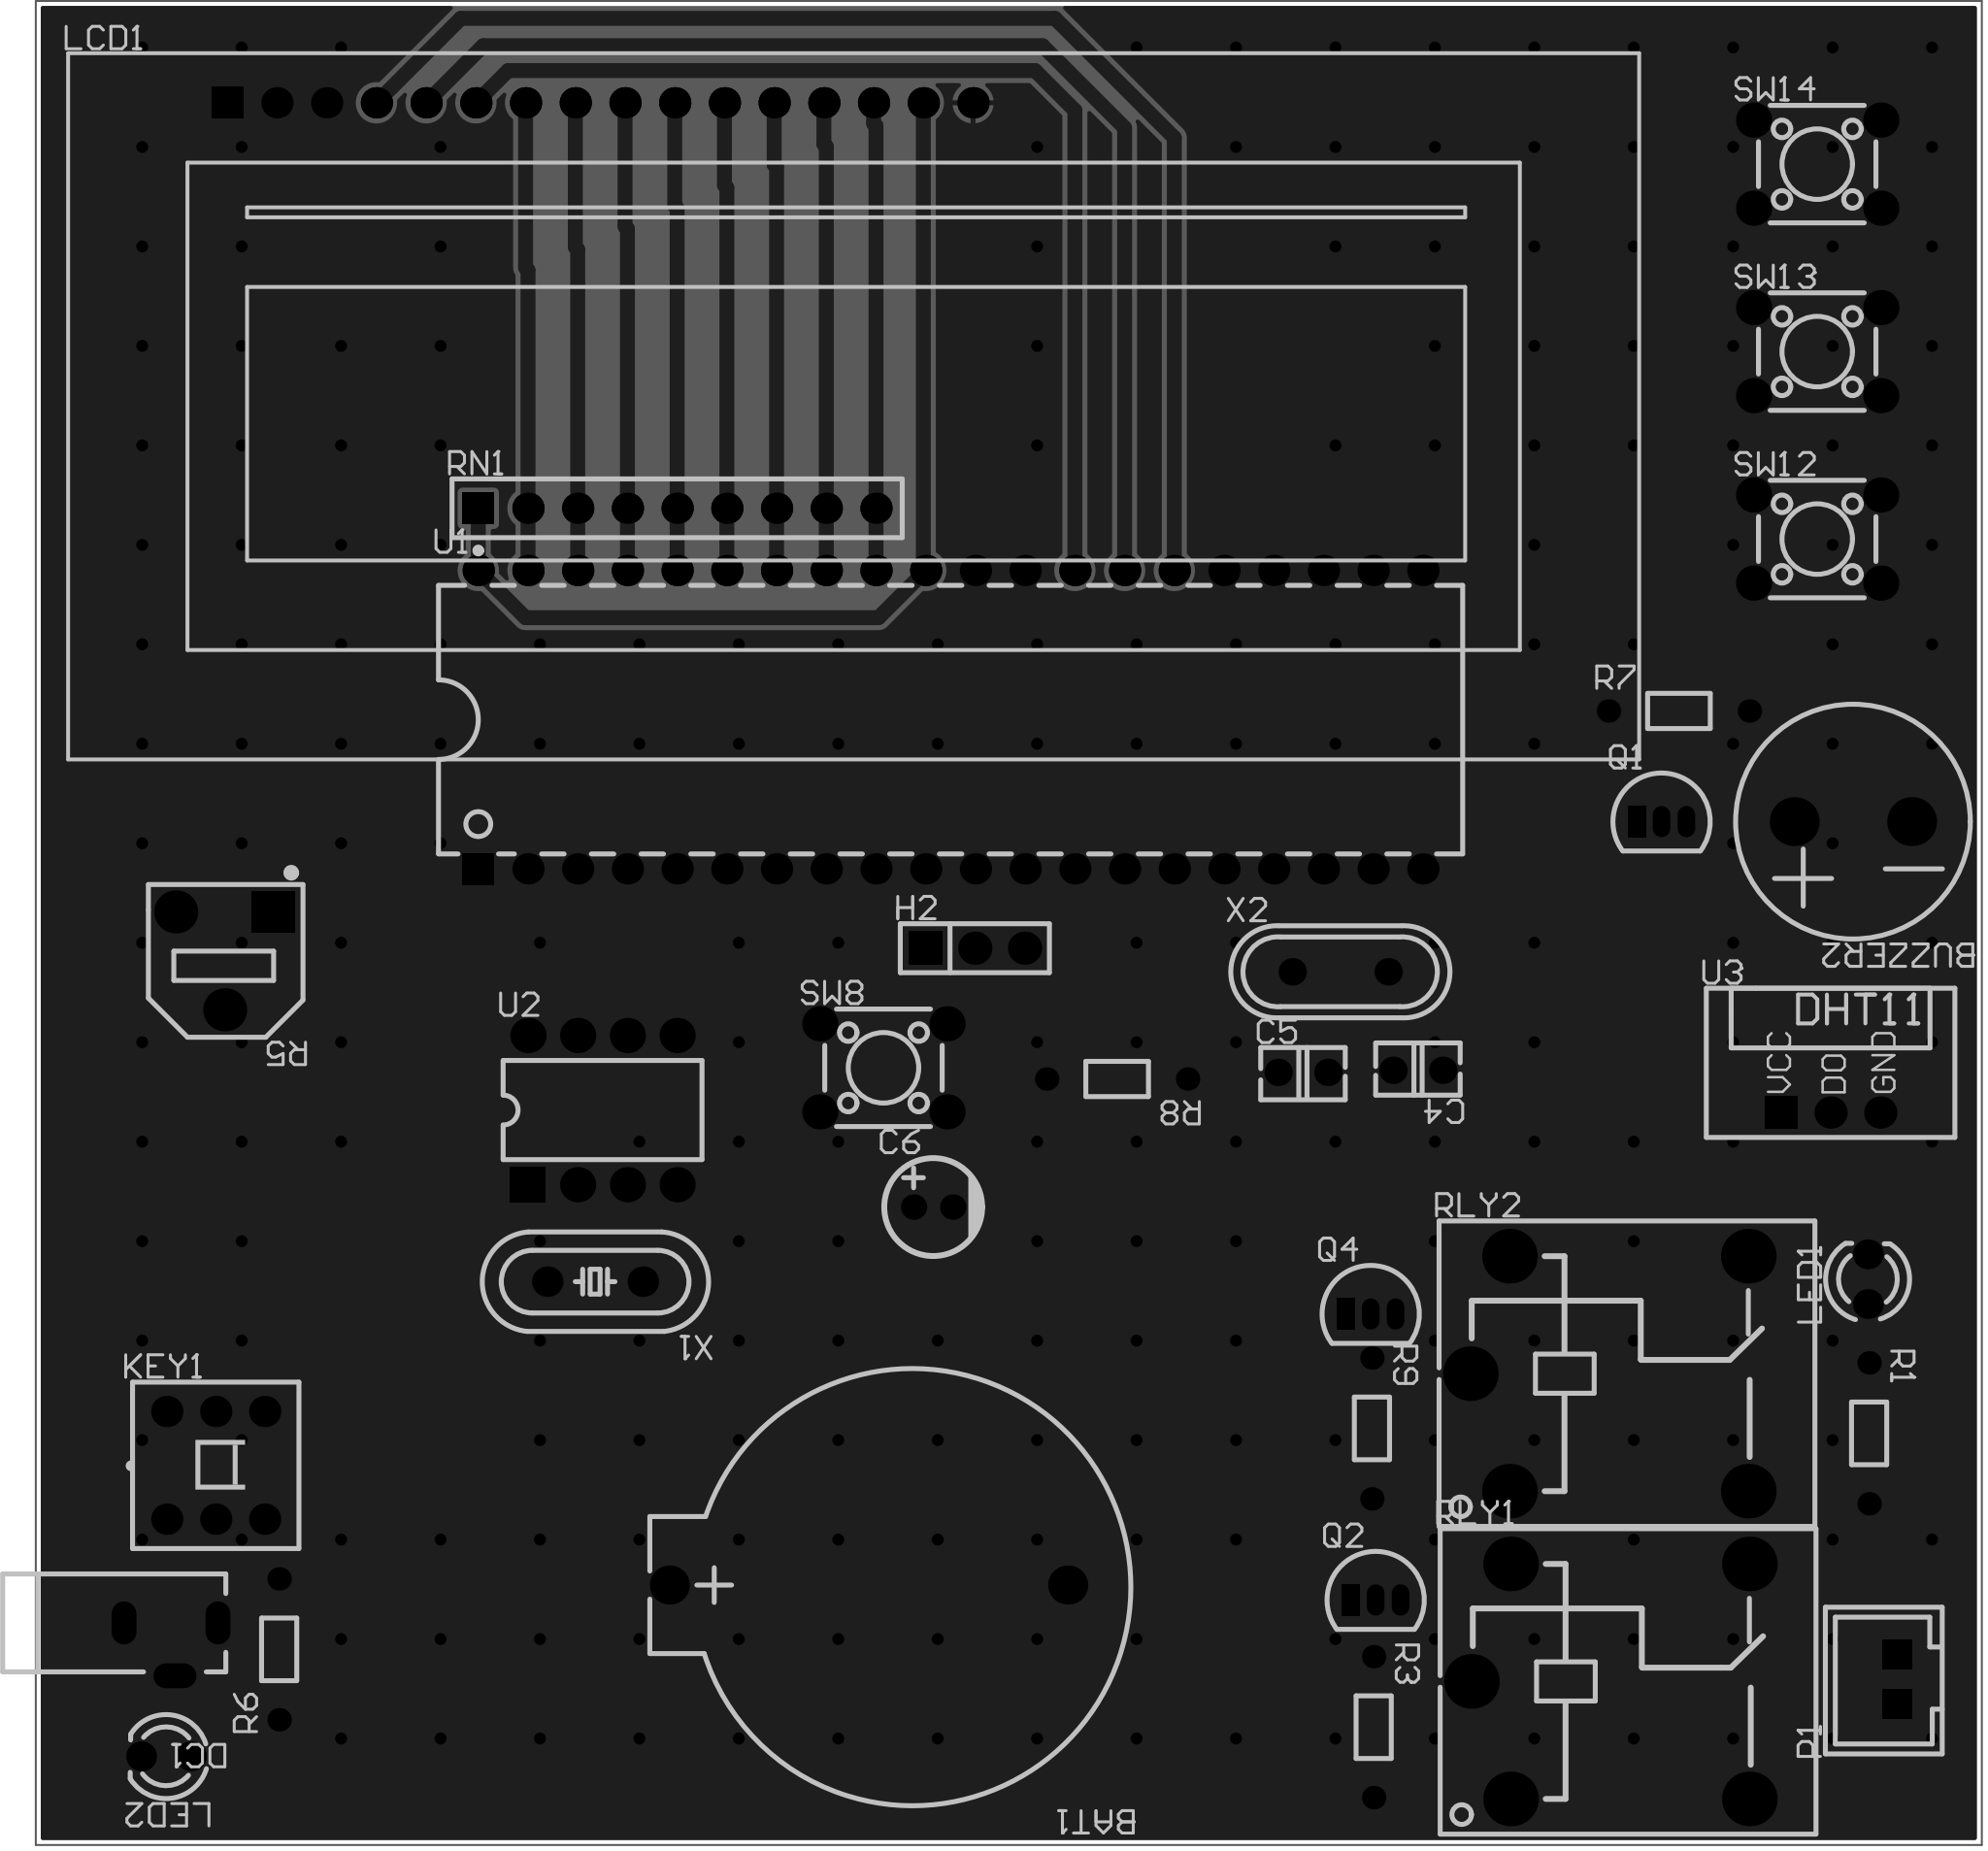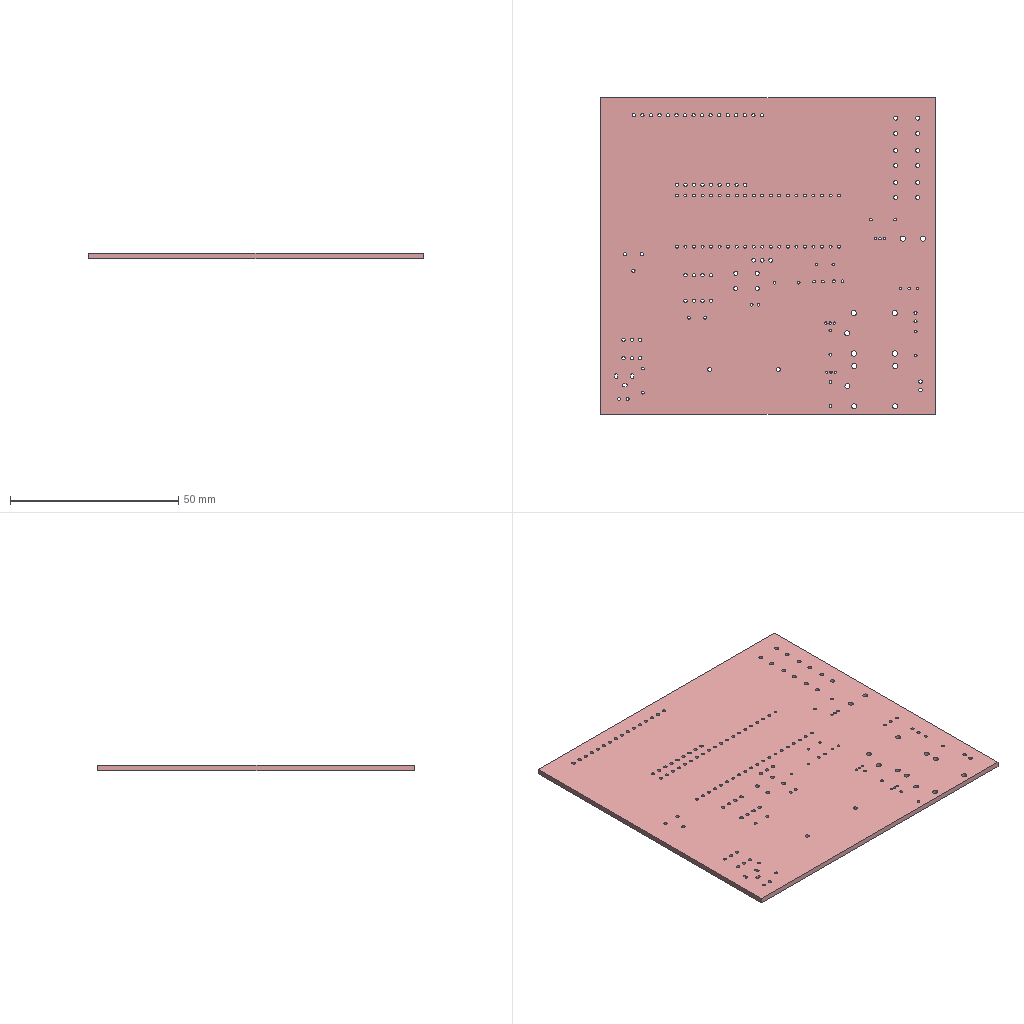Circuit board layout | Altium Designer | box 99.4 x 94.2 x 1.6 mm
Layer stack:
# Altium Designer layer stack of  (unit mm; dielectric type: 0 none, 1 core, 2 prepreg, 3 surface material)
index,name,kind,layer,copper_thickness_mm,dielectric_type,dielectric_thickness_mm,dielectric_material,dielectric_constant
0,Top Paste Mask Layer,other,,,,,,
1,Top Silkscreen Layer,other,,,,,,
2,Top Solder Mask Layer,dielectric,,,3,0.01,,3.3
3,Top Layer,copper,Top Layer,0.035,,,,
4,Dielectric1,dielectric,,,3,1.51,FR4,4.5
5,Bottom Layer,copper,Bottom Layer,0.035,,,,
6,Bottom Solder Mask Layer,dielectric,,,3,0.01,,3.3
7,Bottom Silkscreen Layer,other,,,,,,
8,Bottom Paste Mask Layer,other,,,,,,
# drill layer pairs: low layer,high layer
drill_pair,Top Layer,Bottom Layer
Part placement:
Designator,Comment,Layer,Footprint,Center-X(mm),Center-Y(mm),Rotation
BUZZER2,buzzer,TopLayer,BUZ-TH_BD12.0-P6.00-D0.9-RD,177.546,140.081,180
C4,30pF,TopLayer,CAP-TH_L3.8-W2.5-P2.54-D0.50,155.321,127.381,180
C5,30pF,TopLayer,CAP-TH_L3.8-W2.5-P2.54-D0.50,149.449,127.272,0
C6,10uF,TopLayer,CAP-TH_BD5.0-P2.00-D0.8-FD-10UF50VC110GL,130.556,120.396,0
H2,,TopLayer,HDR-TH_3P-P2.54-V-M,132.685,133.616,0
KEY1,无自锁开关 8.5×8.5 无声,TopLayer,SW-TH_6P-L8.5-W8.5-P2.54,93.903,107.206,0
LCD1,LCD1602,TopLayer,LCD1602,113.542,176.79,0
LED2,,TopLayer,LED_TH-3mm,91.363,92.347,180
Q4,,TopLayer,S8550P_TO-92,152.908,114.935,0
R7,300Ω,TopLayer,Res_1/8W,168.656,145.732,0
R8,10kΩ,TopLayer,Res_1/8W,139.954,126.937,180
R9,1kΩ,TopLayer,Res_1/8W,152.971,109.093,270
R5,10kΩ,TopLayer,RES-ADJ-SMD_RM065-V1,94.361,132.969,180
R6,1kΩ,TopLayer,Res_1/8W,97.142,97.808,90
RLY2,SRD-05VDC-SL-C,TopLayer,RELAY-TH_SRD-XXVDC-XL-C,165.1,111.887,0
SW8,,TopLayer,SW-TH_4P-L6.0-W6.0-P4.50-LS6.5,128.016,127.508,0
SW12,,TopLayer,SW-TH_4P-L6.0-W6.0-P4.50-LS6.5,175.72,154.511,0
SW13,,TopLayer,SW-TH_4P-L6.0-W6.0-P4.50-LS6.5,175.72,164.084,0
SW14,,TopLayer,SW-TH_4P-L6.0-W6.0-P4.50-LS6.5,175.72,173.657,0
U1,STC89C52RC-40I-PDIP40,TopLayer,DIP-40_L52.0-W13.7-P2.54-LS15.2-BL,131.445,145.288,0
X2,11.059MHz,TopLayer,OSC-TH_L11.1-W4.7-P4.88,151.354,132.411,0
DC1,DC-002,TopLayer,DC-IN-TH_DC-3510,91.617,97.808,180
RN1,-,TopLayer,RES-ARRAY-TH_9P-P2.54-D1.0,117.475,156.083,0
BAT1,CR2032-2-1,TopLayer,BAT-TH_CR2032-2-1,127.254,101.092,180
LED1,,TopLayer,LED_TH-3mm,178.308,116.713,90
P1,XH2.54直插座-2P,TopLayer,CONN-TH_XH2.54-2P,179.82,96.277,90
Q2,,TopLayer,S8550P_TO-92,153.162,100.33,0
R1,300Ω,TopLayer,Res_1/8W,178.371,108.839,270
R3,1kΩ,TopLayer,Res_1/8W,153.06,93.835,270
RLY1,SRD-05VDC-SL-C,TopLayer,RELAY-TH_SRD-XXVDC-XL-C,165.155,96.17,0
U2,DS1302N,TopLayer,DIP-8_L9.7-W6.4-P2.54-LS7.6-BL,113.665,125.349,0
U3,DHT11,TopLayer,DHT11_X,176.403,125.222,0
X1,32.768HZ,TopLayer,HC-49S_L11.5-W5.0-P4.88,113.284,116.586,180
Q1,,TopLayer,S8550P_TO-92,167.767,140.081,0
Pad and via stacks:
# Altium Designer via and pad stacks of  (unit mm). Each distinct definition once, with the count of objects using it.
# via: kind,start_layer,end_layer,hole_mm,diameter_mm,mode(0 simple;1 top-mid-bottom;2 full stack),diameter_per_layer,count,example_net
# pad: kind,layer,hole_mm,hole_type(0 round;1 square;2 slot),plating,top_size,top_shape(1 round;2 rect;3 octagon;9 rounded rect),mid_size,bottom_size,mode,footprint,size_per_layer,count,example
pad,Multi-Layer,1.5,0,plated,2.5x2.5,1,2.5x2.5,2.5x2.5,0,BUZ-TH_BD12.0-P6.00-D0.9-RD,,2,BUZZER2.1
pad,Multi-Layer,0.8,0,plated,1.4x1.4,1,1.4x1.4,1.4x1.4,0,CAP-TH_L3.8-W2.5-P2.54-D0.50,,4,C4.1
pad,Multi-Layer,0.8,0,plated,1.3x1.3,1,1.3x1.3,1.3x1.3,0,CAP-TH_BD5.0-P2.00-D0.8-FD-10UF50VC110GL,,2,C6.2
pad,Multi-Layer,1.1,0,plated,1.7x1.7,2,1.7x1.7,1.7x1.7,0,HDR-TH_3P-P2.54-V-M,,1,H2.1
pad,Multi-Layer,1.1,0,plated,1.7x1.7,1,1.7x1.7,1.7x1.7,0,HDR-TH_3P-P2.54-V-M,,2,H2.2
pad,Multi-Layer,1,0,plated,1.6x1.6,1,1.6x1.6,1.6x1.6,0,SW-TH_6P-L8.5-W8.5-P2.54,,6,KEY1.4
pad,Multi-Layer,1,0,plated,1.6x1.6,1,1.6x1.6,1.6x1.6,0,LCD1602,,15,LCD1.16
pad,Multi-Layer,1,0,plated,1.6x1.6,2,1.6x1.6,1.6x1.6,0,LCD1602,,1,LCD1.1
pad,Multi-Layer,0.9144,0,plated,1.524x1.524,1,1.524x1.524,1.524x1.524,0,LED_TH-3mm,,4,LED2.1
pad,Multi-Layer,0.7,0,plated,0.9x1.6,1,0.9x1.6,0.9x1.6,0,S8550P_TO-92,,6,Q4.3
pad,Multi-Layer,0.7,0,plated,0.9x1.6,2,0.9x1.6,0.9x1.6,0,S8550P_TO-92,,3,Q4.1
pad,Multi-Layer,0.8001,0,plated,1.199x1.199,1,1.199x1.199,1.199x1.199,0,Res_1/8W,,12,R7.1
pad,Multi-Layer,1,0,plated,2.2x2.1,2,2.2x2.1,2.2x2.1,0,RES-ADJ-SMD_RM065-V1,,1,R5.1
pad,Multi-Layer,1,0,plated,2.2x2.2,1,2.2x2.2,2.2x2.2,0,RES-ADJ-SMD_RM065-V1,,2,R5.3
pad,Multi-Layer,1.524,0,plated,2.794x2.794,1,2.794x2.794,2.794x2.794,0,RELAY-TH_SRD-XXVDC-XL-C,,10,RLY2.2
pad,Multi-Layer,1.2,0,plated,1.8x1.8,1,1.8x1.8,1.8x1.8,0,SW-TH_4P-L6.0-W6.0-P4.50-LS6.5,,16,SW8.1
pad,Multi-Layer,0.889,0,plated,1.6x1.6,1,1.6x1.6,1.6x1.6,0,DIP-40_L52.0-W13.7-P2.54-LS15.2-BL,,39,U1.31
pad,Multi-Layer,0.889,0,plated,1.6x1.6,2,1.6x1.6,1.6x1.6,0,DIP-40_L52.0-W13.7-P2.54-LS15.2-BL,,1,U1.1
pad,Multi-Layer,0.7,0,plated,1.4x1.4,1,1.4x1.4,1.4x1.4,0,OSC-TH_L11.1-W4.7-P4.88,,2,X2.1
pad,Multi-Layer,0.8,2,plated,2.2x1.27,1,2.2x1.27,2.2x1.27,0,DC-IN-TH_DC-3510,,3,DC1.3
pad,Multi-Layer,1,0,plated,1.6x1.6,2,1.6x1.6,1.6x1.6,0,RES-ARRAY-TH_9P-P2.54-D1.0,,1,RN1.1
pad,Multi-Layer,1,0,plated,1.6x1.6,1,1.6x1.6,1.6x1.6,0,RES-ARRAY-TH_9P-P2.54-D1.0,,8,RN1.2
pad,Multi-Layer,1.2,0,plated,2x2,1,2x2,2x2,0,BAT-TH_CR2032-2-1,,2,BAT1.2
pad,Multi-Layer,1,2,plated,1.524x1.524,2,1.524x1.524,1.524x1.524,0,CONN-TH_XH2.54-2P,,2,P1.1
pad,Multi-Layer,1,0,plated,1.8x1.8,2,1.8x1.8,1.8x1.8,0,DIP-8_L9.7-W6.4-P2.54-LS7.6-BL,,1,U2.1
pad,Multi-Layer,1,0,plated,1.8x1.8,1,1.8x1.8,1.8x1.8,0,DIP-8_L9.7-W6.4-P2.54-LS7.6-BL,,7,U2.2
pad,Multi-Layer,0.81,0,plated,1.651x1.651,2,1.651x1.651,1.651x1.651,0,DHT11_X,,1,U3.1
pad,Multi-Layer,0.81,0,plated,1.651x1.651,1,1.651x1.651,1.651x1.651,0,DHT11_X,,2,U3.2
pad,Multi-Layer,0.9,0,plated,1.56x1.56,1,1.56x1.56,1.56x1.56,0,HC-49S_L11.5-W5.0-P4.88,,2,X1.1
via,Top Layer,Bottom Layer,0.3048,0.61,0,,236,GND
Copper pours:
name,layer,net,type(0 solid;1 hatched;2 none)
Top Layer-GND,Top Layer,GND,0
Bottom Layer-GND,Bottom Layer,GND,0
Design rules, without the lines most boards share:
# Altium Designer design rules of  (exported by Altium Designer, unit mm)
# columns: name | kind | enabled | priority | scope1 | scope2 | descriptor | typed fields (field=value)
creepage | 65 | enabled | 1 | All | All | Creepage Distance Constraint =(0mil) (All),(All) |
copperRegion | 20 | enabled | 1 | (InNet('GND')) | All | Polygon Connect Rule(Relief Connect )(Conductor Width=10mil) (Relief Angle=90 Angle) (Entries=4) (Air Gap Width=10mil) ((InNet('GND'))),(All) | connect_style(0=relief,1=direct,2=none)=0 relief_conductor_width=0.254 relief_entries=4